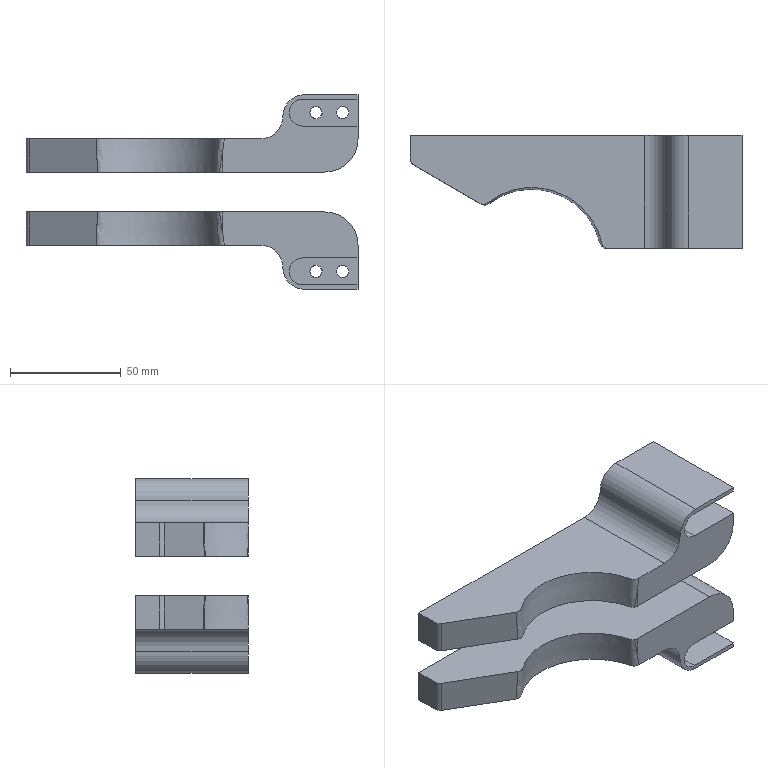Part | 2 solids | 42 faces | box 150 x 51 x 88 mm | volume 215383 mm3 | plane 22 | cylinder 16 | spline 4 | commonest cylinder face diameters 5.5 x4 6 x4 20 x4 12.2 x2 30 x2